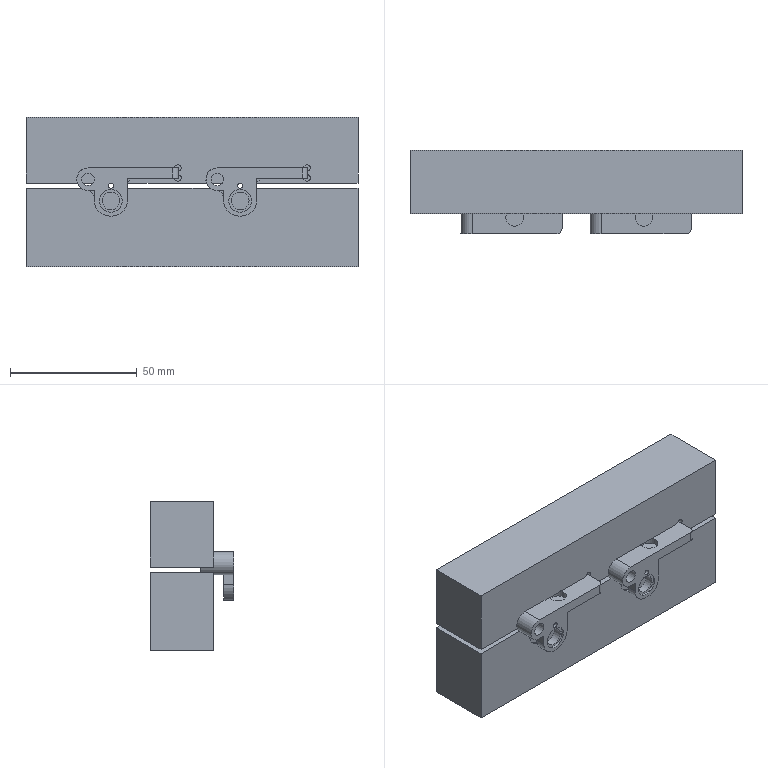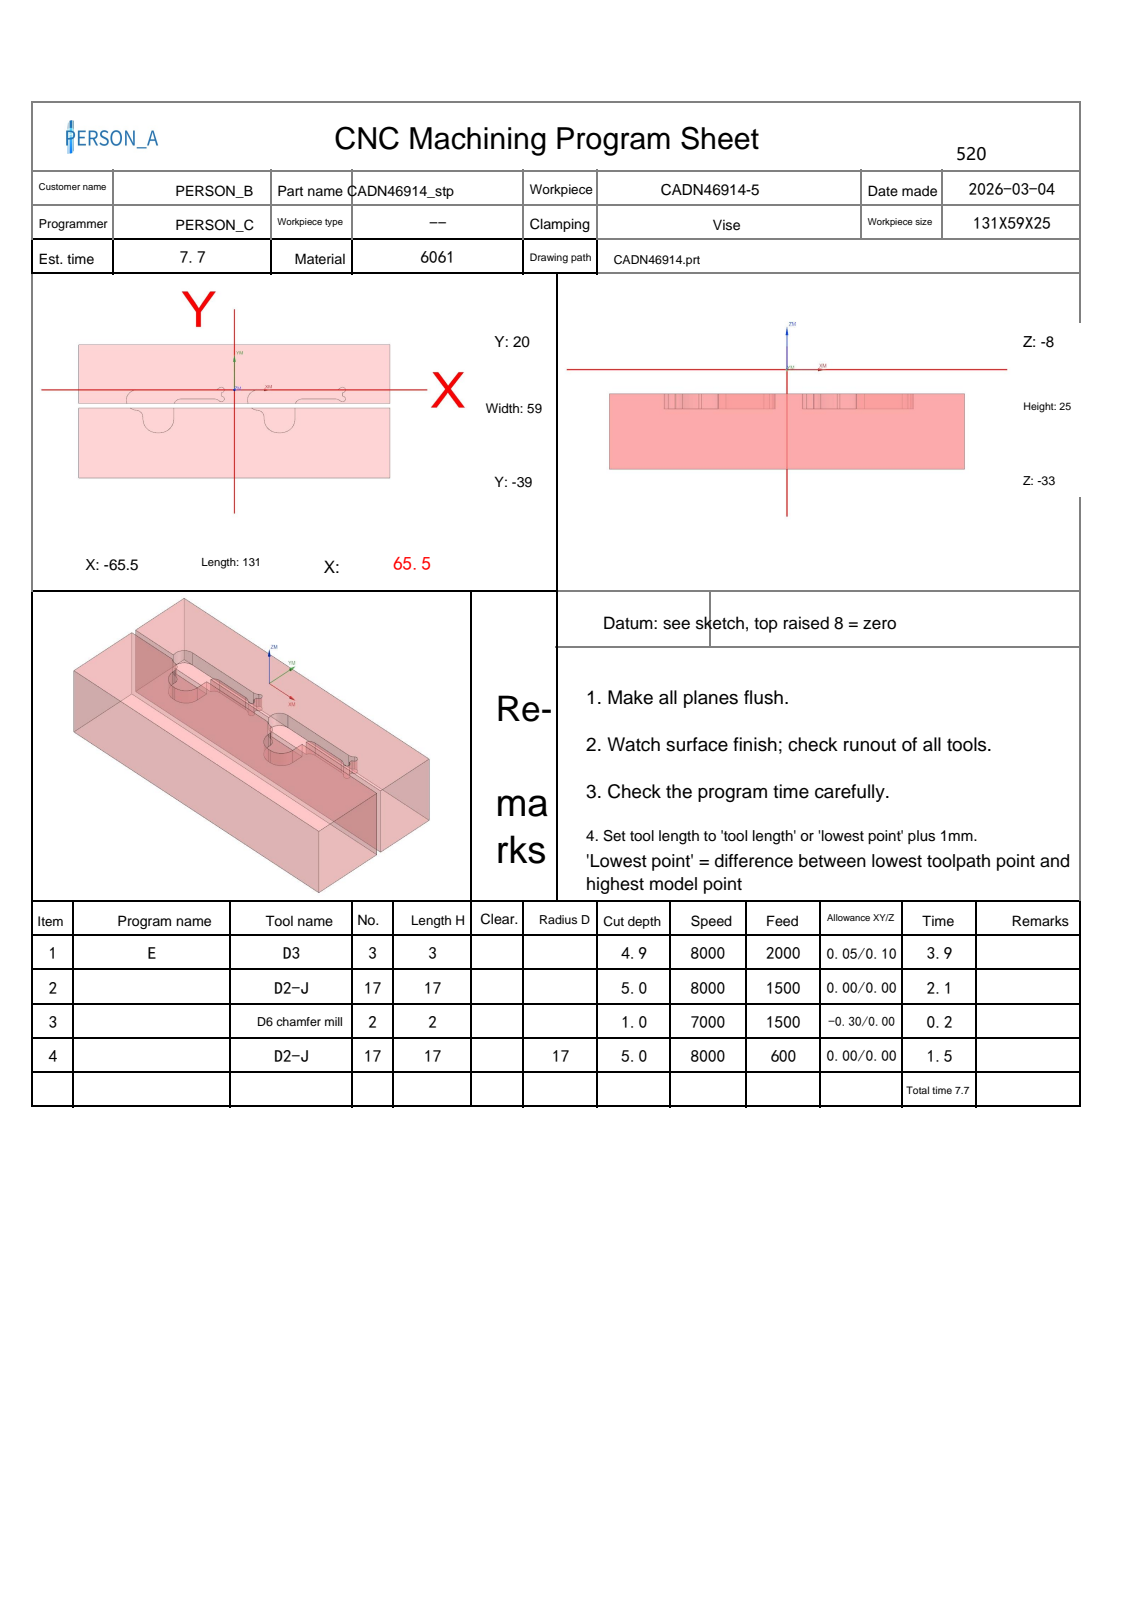NC program | NX | posted by the shop | part box 131 x 33 x 59 mm
Lines 1 to 1054 of 10523:
%
O0001
(Machine time: 8.40 MIN)
(===Total Tool:3===)
(T3=D3      D=3.   R=0.   D-  H03 Z=-12.9 )
(T17=D2-J   D=2.   R=0.   D-  H17 Z=-13.  )
(T2=D6 chamfer mill   D=6.   R=0.   D-  H02 Z=-9.   )
G80 G90 G17 G49 G40
G91 G28 Z0
M01
N1 T03 M06
(D3  D=3. R=0. H=03 ce=0.05 di=0.10)
G00 G90 G54 X-31.564 Y-11.328 M03 S8000
G43 H03 Z2.1
M08
Z-6.5
G03 X-31.564 Y-11.328 Z-6.945 I-1.336 J.192 F2000.
X-31.564 Y-11.328 Z-7.389 I-1.336 J.192
X-31.564 Y-11.328 Z-7.834 I-1.336 J.192
X-31.564 Y-11.328 Z-8.278 I-1.336 J.192
X-31.55 Y-11.136 Z-8.288 I-1.336 J.192
G01 Y-9.622
X-31.538 Y-9.552
X-31.579 Y-9.494
G02 X-32.02 Y-7.55 I4.059 J1.944
X-31.877 Y-6.424 I4.5 J0.0
G01 X-31.868 Y-6.35
G03 X-32.167 Y-6.05 I-.3 J0.0
G01 X-34.038
G03 X-34.338 Y-6.35 I.001 J-.3
G01 X-34.277 Y-6.53
G02 X-32.45 Y-11.983 I-7.223 J-5.453
G01 Y-12.651
G03 X-32.151 Y-12.95 I.3 J.001
G01 X-31.849
G03 X-31.55 Y-12.651 I-.001 J.3
G01 Y-12.047
G02 X-31.417 Y-11.797 I.3 J0.0
G01 X-29.433 Y-10.475
G03 X-29.3 Y-10.226 I-.167 J.25
G01 Y-9.025
X-29.295 Y-8.929
X-29.355 Y-8.853
G02 X-29.77 Y-7.55 I1.835 J1.303
X-29.642 Y-6.8 I2.25 J0.0
G01 X-29.183 Y-5.502
X-29.15 Y-5.439
X-29.154 Y-5.369
X-29.196 Y-5.311
X-29.331 Y-5.049
X-29.376 Y-4.983
X-29.363 Y-4.904
Y-4.886
G03 X-30.113 Y-4.136 I-.75 J0.0
X-30.544 Y-4.272 I0.0 J-.75
G01 X-31.725 Y-5.102
G03 X-32.044 Y-5.716 I.431 J-.614
X-31.294 Y-6.466 I.75 J0.0
X-30.863 Y-6.329 I0.0 J.75
G01 X-29.682 Y-5.5
G03 X-29.512 Y-5.334 I-.431 J.614
G01 X-29.481 Y-5.274
X-29.416 Y-5.258
X-29.155 Y-5.143
G03 X-28.994 Y-4.968 I-.122 J.274
G01 X-28.911 Y-4.733
G02 X-28.707 Y-4.222 I6.411 J-2.267
G01 X-28.681 Y-4.1
G03 X-28.98 Y-3.8 I-.3 J0.0
G01 X-36.616
G03 X-36.82 Y-3.881 I0.0 J-.3
G01 X-37.21 Y-4.244
X-37.275 Y-4.313
X-37.37 Y-4.321
G03 X-38.008 Y-5.063 I.111 J-.742
X-37.505 Y-5.771 I.75 J0.0
G01 X-35.247 Y-6.558
G03 X-35. Y-6.6 I.247 J.708
X-34.25 Y-5.85 I0.0 J.75
X-34.753 Y-5.142 I-.75 J0.0
G01 X-36.671 Y-4.473
X-36.754 Y-4.453
X-36.803 Y-4.382
X-37.199 Y-3.908
G03 X-37.429 Y-3.8 I-.23 J-.192
G01 X-41.
G03 X-41.7 Y-4.5 I0.0 J-.7
X-41.66 Y-4.733 I.7 J0.0
G01 X-41.622 Y-4.841
X-41.601 Y-4.925
X-41.529 Y-4.973
X-41.44 Y-5.044
G03 X-41.047 Y-5.198 I.44 J.544
G02 X-34.7 Y-11.983 I-.453 J-6.785
G01 Y-13.
G03 X-32.5 Y-15.2 I2.2 J0.0
G01 X-31.5
G03 X-29.3 Y-13. I0.0 J2.2
G01 Y-12.047
G02 X-29.167 Y-11.797 I.3 J0.0
G01 X-27.183 Y-10.475
G03 X-27.05 Y-10.226 I-.167 J.25
G01 Y-7.55
X-27.52
X-26.79 Y-5.483
G02 X-22.5 Y-2.45 I4.29 J-1.517
G01 X-8.51
G02 X-7.05 Y-2.691 I0.0 J-4.55
G01 Y-1.309
G02 X-8.51 Y-1.55 I-1.46 J4.309
G01 X-26.738
G03 X-27.038 Y-1.85 I0.0 J-.3
G01 X-27.031 Y-1.913
X-27.025 Y-1.94
X-27.018 Y-2.004
G02 X-27.194 Y-2.277 I-.3 J0.0
G01 X-28.386 Y-2.819
G03 X-28.825 Y-3.502 I.311 J-.683
X-28.075 Y-4.252 I.75 J0.0
X-27.765 Y-4.184 I0.0 J.75
G01 X-26.117 Y-3.434
G03 X-25.677 Y-2.752 I-.311 J.683
X-26.318 Y-2.01 I-.75 J0.0
G02 X-26.544 Y-1.813 I.041 J.275
G01 X-26.589 Y-1.662
X-26.605 Y-1.591
X-26.665 Y-1.546
X-26.738 Y-1.55
X-41.
G03 X-43.95 Y-4.5 I0.0 J-2.95
X-43.781 Y-5.483 I2.95 J0.0
G01 X-43.44 Y-6.45
X-43.28
X-42.854 Y-6.794
G03 X-41.197 Y-7.443 I1.854 J2.294
G02 X-36.95 Y-11.983 I-.303 J-4.54
G01 Y-13.
G03 X-32.5 Y-17.45 I4.45 J0.0
G01 X-31.5
G03 X-27.05 Y-13. I0.0 J4.45
G01 Y-9.636
Y-9.136
X-30.05
Z-6.788
G00 X-31.564 Y-11.328
G03 X-31.564 Y-11.328 Z-7.233 I-1.336 J.192
X-31.564 Y-11.328 Z-7.677 I-1.336 J.192
X-31.564 Y-11.328 Z-8.122 I-1.336 J.192
X-31.564 Y-11.328 Z-8.566 I-1.336 J.192
X-31.55 Y-11.136 Z-8.576 I-1.336 J.192
G01 Y-9.622
X-31.538 Y-9.552
X-31.579 Y-9.494
G02 X-32.02 Y-7.55 I4.059 J1.944
X-31.877 Y-6.424 I4.5 J0.0
G01 X-31.868 Y-6.35
G03 X-32.167 Y-6.05 I-.3 J0.0
G01 X-34.038
G03 X-34.338 Y-6.35 I.001 J-.3
G01 X-34.277 Y-6.53
G02 X-32.45 Y-11.983 I-7.223 J-5.453
G01 Y-12.651
G03 X-32.151 Y-12.95 I.3 J.001
G01 X-31.849
G03 X-31.55 Y-12.651 I-.001 J.3
G01 Y-12.047
G02 X-31.417 Y-11.797 I.3 J0.0
G01 X-29.433 Y-10.475
G03 X-29.3 Y-10.226 I-.167 J.25
G01 Y-9.025
X-29.295 Y-8.929
X-29.355 Y-8.853
G02 X-29.77 Y-7.55 I1.835 J1.303
X-29.642 Y-6.8 I2.25 J0.0
G01 X-29.183 Y-5.502
X-29.15 Y-5.439
X-29.154 Y-5.369
X-29.196 Y-5.311
X-29.331 Y-5.049
X-29.376 Y-4.983
X-29.363 Y-4.904
Y-4.886
G03 X-30.113 Y-4.136 I-.75 J0.0
X-30.544 Y-4.272 I0.0 J-.75
G01 X-31.725 Y-5.102
G03 X-32.044 Y-5.716 I.431 J-.614
X-31.294 Y-6.466 I.75 J0.0
X-30.863 Y-6.329 I0.0 J.75
G01 X-29.682 Y-5.5
G03 X-29.512 Y-5.334 I-.431 J.614
G01 X-29.481 Y-5.274
X-29.416 Y-5.258
X-29.155 Y-5.143
G03 X-28.994 Y-4.968 I-.122 J.274
G01 X-28.911 Y-4.733
G02 X-28.707 Y-4.222 I6.411 J-2.267
G01 X-28.681 Y-4.1
G03 X-28.98 Y-3.8 I-.3 J0.0
G01 X-36.616
G03 X-36.82 Y-3.881 I0.0 J-.3
G01 X-37.21 Y-4.244
X-37.275 Y-4.313
X-37.37 Y-4.321
G03 X-38.008 Y-5.063 I.111 J-.742
X-37.505 Y-5.771 I.75 J0.0
G01 X-35.247 Y-6.558
G03 X-35. Y-6.6 I.247 J.708
X-34.25 Y-5.85 I0.0 J.75
X-34.753 Y-5.142 I-.75 J0.0
G01 X-36.671 Y-4.473
X-36.754 Y-4.453
X-36.803 Y-4.382
X-37.199 Y-3.908
G03 X-37.429 Y-3.8 I-.23 J-.192
G01 X-41.
G03 X-41.7 Y-4.5 I0.0 J-.7
X-41.66 Y-4.733 I.7 J0.0
G01 X-41.622 Y-4.841
X-41.601 Y-4.925
X-41.529 Y-4.973
X-41.44 Y-5.044
G03 X-41.047 Y-5.198 I.44 J.544
G02 X-34.7 Y-11.983 I-.453 J-6.785
G01 Y-13.
G03 X-32.5 Y-15.2 I2.2 J0.0
G01 X-31.5
G03 X-29.3 Y-13. I0.0 J2.2
G01 Y-12.047
G02 X-29.167 Y-11.797 I.3 J0.0
G01 X-27.183 Y-10.475
G03 X-27.05 Y-10.226 I-.167 J.25
G01 Y-7.55
X-27.52
X-26.79 Y-5.483
G02 X-22.5 Y-2.45 I4.29 J-1.517
G01 X-8.51
G02 X-7.05 Y-2.691 I0.0 J-4.55
G01 Y-1.309
G02 X-8.51 Y-1.55 I-1.46 J4.309
G01 X-26.738
G03 X-27.038 Y-1.85 I0.0 J-.3
G01 X-27.031 Y-1.913
X-27.025 Y-1.94
X-27.018 Y-2.004
G02 X-27.194 Y-2.277 I-.3 J0.0
G01 X-28.386 Y-2.819
G03 X-28.825 Y-3.502 I.311 J-.683
X-28.075 Y-4.252 I.75 J0.0
X-27.765 Y-4.184 I0.0 J.75
G01 X-26.117 Y-3.434
G03 X-25.677 Y-2.752 I-.311 J.683
X-26.318 Y-2.01 I-.75 J0.0
G02 X-26.544 Y-1.813 I.041 J.275
G01 X-26.589 Y-1.662
X-26.605 Y-1.591
X-26.665 Y-1.546
X-26.738 Y-1.55
X-41.
G03 X-43.95 Y-4.5 I0.0 J-2.95
X-43.781 Y-5.483 I2.95 J0.0
G01 X-43.44 Y-6.45
X-43.28
X-42.854 Y-6.794
G03 X-41.197 Y-7.443 I1.854 J2.294
G02 X-36.95 Y-11.983 I-.303 J-4.54
G01 Y-13.
G03 X-32.5 Y-17.45 I4.45 J0.0
G01 X-31.5
G03 X-27.05 Y-13. I0.0 J4.45
G01 Y-9.636
Y-9.136
X-30.05
Z-7.076
G00 X-31.564 Y-11.328
G03 X-31.564 Y-11.328 Z-7.521 I-1.336 J.192
X-31.564 Y-11.328 Z-7.966 I-1.336 J.192
X-31.564 Y-11.328 Z-8.41 I-1.336 J.192
X-31.564 Y-11.328 Z-8.855 I-1.336 J.192
X-31.55 Y-11.136 Z-8.865 I-1.336 J.192
G01 Y-9.622
X-31.538 Y-9.552
X-31.579 Y-9.494
G02 X-32.02 Y-7.55 I4.059 J1.944
X-31.877 Y-6.424 I4.5 J0.0
G01 X-31.868 Y-6.35
G03 X-32.167 Y-6.05 I-.3 J0.0
G01 X-34.038
G03 X-34.338 Y-6.35 I.001 J-.3
G01 X-34.277 Y-6.53
G02 X-32.45 Y-11.983 I-7.223 J-5.453
G01 Y-12.651
G03 X-32.151 Y-12.95 I.3 J.001
G01 X-31.849
G03 X-31.55 Y-12.651 I-.001 J.3
G01 Y-12.047
G02 X-31.417 Y-11.797 I.3 J0.0
G01 X-29.433 Y-10.475
G03 X-29.3 Y-10.226 I-.167 J.25
G01 Y-9.025
X-29.295 Y-8.929
X-29.355 Y-8.853
G02 X-29.77 Y-7.55 I1.835 J1.303
X-29.642 Y-6.8 I2.25 J0.0
G01 X-29.183 Y-5.502
X-29.15 Y-5.439
X-29.154 Y-5.369
X-29.196 Y-5.311
X-29.331 Y-5.049
X-29.376 Y-4.983
X-29.363 Y-4.904
Y-4.886
G03 X-30.113 Y-4.136 I-.75 J0.0
X-30.544 Y-4.272 I0.0 J-.75
G01 X-31.725 Y-5.102
G03 X-32.044 Y-5.716 I.431 J-.614
X-31.294 Y-6.466 I.75 J0.0
X-30.863 Y-6.329 I0.0 J.75
G01 X-29.682 Y-5.5
G03 X-29.512 Y-5.334 I-.431 J.614
G01 X-29.481 Y-5.274
X-29.416 Y-5.258
X-29.155 Y-5.143
G03 X-28.994 Y-4.968 I-.122 J.274
G01 X-28.911 Y-4.733
G02 X-28.707 Y-4.222 I6.411 J-2.267
G01 X-28.681 Y-4.1
G03 X-28.98 Y-3.8 I-.3 J0.0
G01 X-36.616
G03 X-36.82 Y-3.881 I0.0 J-.3
G01 X-37.21 Y-4.244
X-37.275 Y-4.313
X-37.37 Y-4.321
G03 X-38.008 Y-5.063 I.111 J-.742
X-37.505 Y-5.771 I.75 J0.0
G01 X-35.247 Y-6.558
G03 X-35. Y-6.6 I.247 J.708
X-34.25 Y-5.85 I0.0 J.75
X-34.753 Y-5.142 I-.75 J0.0
G01 X-36.671 Y-4.473
X-36.754 Y-4.453
X-36.803 Y-4.382
X-37.199 Y-3.908
G03 X-37.429 Y-3.8 I-.23 J-.192
G01 X-41.
G03 X-41.7 Y-4.5 I0.0 J-.7
X-41.66 Y-4.733 I.7 J0.0
G01 X-41.622 Y-4.841
X-41.601 Y-4.925
X-41.529 Y-4.973
X-41.44 Y-5.044
G03 X-41.047 Y-5.198 I.44 J.544
G02 X-34.7 Y-11.983 I-.453 J-6.785
G01 Y-13.
G03 X-32.5 Y-15.2 I2.2 J0.0
G01 X-31.5
G03 X-29.3 Y-13. I0.0 J2.2
G01 Y-12.047
G02 X-29.167 Y-11.797 I.3 J0.0
G01 X-27.183 Y-10.475
G03 X-27.05 Y-10.226 I-.167 J.25
G01 Y-7.55
X-27.52
X-26.79 Y-5.483
G02 X-22.5 Y-2.45 I4.29 J-1.517
G01 X-8.51
G02 X-7.05 Y-2.691 I0.0 J-4.55
G01 Y-1.309
G02 X-8.51 Y-1.55 I-1.46 J4.309
G01 X-26.738
G03 X-27.038 Y-1.85 I0.0 J-.3
G01 X-27.031 Y-1.913
X-27.025 Y-1.94
X-27.018 Y-2.004
G02 X-27.194 Y-2.277 I-.3 J0.0
G01 X-28.386 Y-2.819
G03 X-28.825 Y-3.502 I.311 J-.683
X-28.075 Y-4.252 I.75 J0.0
X-27.765 Y-4.184 I0.0 J.75
G01 X-26.117 Y-3.434
G03 X-25.677 Y-2.752 I-.311 J.683
X-26.318 Y-2.01 I-.75 J0.0
G02 X-26.544 Y-1.813 I.041 J.275
G01 X-26.589 Y-1.662
X-26.605 Y-1.591
X-26.665 Y-1.546
X-26.738 Y-1.55
X-41.
G03 X-43.95 Y-4.5 I0.0 J-2.95
X-43.781 Y-5.483 I2.95 J0.0
G01 X-43.44 Y-6.45
X-43.28
X-42.854 Y-6.794
G03 X-41.197 Y-7.443 I1.854 J2.294
G02 X-36.95 Y-11.983 I-.303 J-4.54
G01 Y-13.
G03 X-32.5 Y-17.45 I4.45 J0.0
G01 X-31.5
G03 X-27.05 Y-13. I0.0 J4.45
G01 Y-9.636
Y-9.136
X-30.05
Z-7.365
G00 X-31.564 Y-11.328
G03 X-31.564 Y-11.328 Z-7.809 I-1.336 J.192
X-31.564 Y-11.328 Z-8.254 I-1.336 J.192
X-31.564 Y-11.328 Z-8.698 I-1.336 J.192
X-31.564 Y-11.328 Z-9.143 I-1.336 J.192
X-31.55 Y-11.136 Z-9.153 I-1.336 J.192
G01 Y-9.622
X-31.538 Y-9.552
X-31.579 Y-9.494
G02 X-32.02 Y-7.55 I4.059 J1.944
X-31.877 Y-6.424 I4.5 J0.0
G01 X-31.868 Y-6.35
G03 X-32.167 Y-6.05 I-.3 J0.0
G01 X-34.038
G03 X-34.338 Y-6.35 I.001 J-.3
G01 X-34.277 Y-6.53
G02 X-32.45 Y-11.983 I-7.223 J-5.453
G01 Y-12.651
G03 X-32.151 Y-12.95 I.3 J.001
G01 X-31.849
G03 X-31.55 Y-12.651 I-.001 J.3
G01 Y-12.047
G02 X-31.417 Y-11.797 I.3 J0.0
G01 X-29.433 Y-10.475
G03 X-29.3 Y-10.226 I-.167 J.25
G01 Y-9.025
X-29.295 Y-8.929
X-29.355 Y-8.853
G02 X-29.77 Y-7.55 I1.835 J1.303
X-29.642 Y-6.8 I2.25 J0.0
G01 X-29.183 Y-5.502
X-29.15 Y-5.439
X-29.154 Y-5.369
X-29.196 Y-5.311
X-29.331 Y-5.049
X-29.376 Y-4.983
X-29.363 Y-4.904
Y-4.886
G03 X-30.113 Y-4.136 I-.75 J0.0
X-30.544 Y-4.272 I0.0 J-.75
G01 X-31.725 Y-5.102
G03 X-32.044 Y-5.716 I.431 J-.614
X-31.294 Y-6.466 I.75 J0.0
X-30.863 Y-6.329 I0.0 J.75
G01 X-29.682 Y-5.5
G03 X-29.512 Y-5.334 I-.431 J.614
G01 X-29.481 Y-5.274
X-29.416 Y-5.258
X-29.155 Y-5.143
G03 X-28.994 Y-4.968 I-.122 J.274
G01 X-28.911 Y-4.733
G02 X-28.707 Y-4.222 I6.411 J-2.267
G01 X-28.681 Y-4.1
G03 X-28.98 Y-3.8 I-.3 J0.0
G01 X-36.616
G03 X-36.82 Y-3.881 I0.0 J-.3
G01 X-37.21 Y-4.244
X-37.275 Y-4.313
X-37.37 Y-4.321
G03 X-38.008 Y-5.063 I.111 J-.742
X-37.505 Y-5.771 I.75 J0.0
G01 X-35.247 Y-6.558
G03 X-35. Y-6.6 I.247 J.708
X-34.25 Y-5.85 I0.0 J.75
X-34.753 Y-5.142 I-.75 J0.0
G01 X-36.671 Y-4.473
X-36.754 Y-4.453
X-36.803 Y-4.382
X-37.199 Y-3.908
G03 X-37.429 Y-3.8 I-.23 J-.192
G01 X-41.
G03 X-41.7 Y-4.5 I0.0 J-.7
X-41.66 Y-4.733 I.7 J0.0
G01 X-41.622 Y-4.841
X-41.601 Y-4.925
X-41.529 Y-4.973
X-41.44 Y-5.044
G03 X-41.047 Y-5.198 I.44 J.544
G02 X-34.7 Y-11.983 I-.453 J-6.785
G01 Y-13.
G03 X-32.5 Y-15.2 I2.2 J0.0
G01 X-31.5
G03 X-29.3 Y-13. I0.0 J2.2
G01 Y-12.047
G02 X-29.167 Y-11.797 I.3 J0.0
G01 X-27.183 Y-10.475
G03 X-27.05 Y-10.226 I-.167 J.25
G01 Y-7.55
X-27.52
X-26.79 Y-5.483
G02 X-22.5 Y-2.45 I4.29 J-1.517
G01 X-8.51
G02 X-7.05 Y-2.691 I0.0 J-4.55
G01 Y-1.309
G02 X-8.51 Y-1.55 I-1.46 J4.309
G01 X-26.738
G03 X-27.038 Y-1.85 I0.0 J-.3
G01 X-27.031 Y-1.913
X-27.025 Y-1.94
X-27.018 Y-2.004
G02 X-27.194 Y-2.277 I-.3 J0.0
G01 X-28.386 Y-2.819
G03 X-28.825 Y-3.502 I.311 J-.683
X-28.075 Y-4.252 I.75 J0.0
X-27.765 Y-4.184 I0.0 J.75
G01 X-26.117 Y-3.434
G03 X-25.677 Y-2.752 I-.311 J.683
X-26.318 Y-2.01 I-.75 J0.0
G02 X-26.544 Y-1.813 I.041 J.275
G01 X-26.589 Y-1.662
X-26.605 Y-1.591
X-26.665 Y-1.546
X-26.738 Y-1.55
X-41.
G03 X-43.95 Y-4.5 I0.0 J-2.95
X-43.781 Y-5.483 I2.95 J0.0
G01 X-43.44 Y-6.45
X-43.28
X-42.854 Y-6.794
G03 X-41.197 Y-7.443 I1.854 J2.294
G02 X-36.95 Y-11.983 I-.303 J-4.54
G01 Y-13.
G03 X-32.5 Y-17.45 I4.45 J0.0
G01 X-31.5
G03 X-27.05 Y-13. I0.0 J4.45
G01 Y-9.636
Y-9.136
X-30.05
Z-7.653
G00 X-31.564 Y-11.328
G03 X-31.564 Y-11.328 Z-8.097 I-1.336 J.192
X-31.564 Y-11.328 Z-8.542 I-1.336 J.192
X-31.564 Y-11.328 Z-8.987 I-1.336 J.192
X-31.564 Y-11.328 Z-9.431 I-1.336 J.192
X-31.55 Y-11.136 Z-9.441 I-1.336 J.192
G01 Y-9.622
X-31.538 Y-9.552
X-31.579 Y-9.494
G02 X-32.02 Y-7.55 I4.059 J1.944
X-31.877 Y-6.424 I4.5 J0.0
G01 X-31.868 Y-6.35
G03 X-32.167 Y-6.05 I-.3 J0.0
G01 X-34.038
G03 X-34.338 Y-6.35 I.001 J-.3
G01 X-34.277 Y-6.53
G02 X-32.45 Y-11.983 I-7.223 J-5.453
G01 Y-12.651
G03 X-32.151 Y-12.95 I.3 J.001
G01 X-31.849
G03 X-31.55 Y-12.651 I-.001 J.3
G01 Y-12.047
G02 X-31.417 Y-11.797 I.3 J0.0
G01 X-29.433 Y-10.475
G03 X-29.3 Y-10.226 I-.167 J.25
G01 Y-9.025
X-29.295 Y-8.929
X-29.355 Y-8.853
G02 X-29.77 Y-7.55 I1.835 J1.303
X-29.642 Y-6.8 I2.25 J0.0
G01 X-29.183 Y-5.502
X-29.15 Y-5.439
X-29.154 Y-5.369
X-29.196 Y-5.311
X-29.331 Y-5.049
X-29.376 Y-4.983
X-29.363 Y-4.904
Y-4.886
G03 X-30.113 Y-4.136 I-.75 J0.0
X-30.544 Y-4.272 I0.0 J-.75
G01 X-31.725 Y-5.102
G03 X-32.044 Y-5.716 I.431 J-.614
X-31.294 Y-6.466 I.75 J0.0
X-30.863 Y-6.329 I0.0 J.75
G01 X-29.682 Y-5.5
G03 X-29.512 Y-5.334 I-.431 J.614
G01 X-29.481 Y-5.274
X-29.416 Y-5.258
X-29.155 Y-5.143
G03 X-28.994 Y-4.968 I-.122 J.274
G01 X-28.911 Y-4.733
G02 X-28.707 Y-4.222 I6.411 J-2.267
G01 X-28.681 Y-4.1
G03 X-28.98 Y-3.8 I-.3 J0.0
G01 X-36.616
G03 X-36.82 Y-3.881 I0.0 J-.3
G01 X-37.21 Y-4.244
X-37.275 Y-4.313
X-37.37 Y-4.321
G03 X-38.008 Y-5.063 I.111 J-.742
X-37.505 Y-5.771 I.75 J0.0
G01 X-35.247 Y-6.558
G03 X-35. Y-6.6 I.247 J.708
X-34.25 Y-5.85 I0.0 J.75
X-34.753 Y-5.142 I-.75 J0.0
G01 X-36.671 Y-4.473
X-36.754 Y-4.453
X-36.803 Y-4.382
X-37.199 Y-3.908
G03 X-37.429 Y-3.8 I-.23 J-.192
G01 X-41.
G03 X-41.7 Y-4.5 I0.0 J-.7
X-41.66 Y-4.733 I.7 J0.0
G01 X-41.622 Y-4.841
X-41.601 Y-4.925
X-41.529 Y-4.973
X-41.44 Y-5.044
G03 X-41.047 Y-5.198 I.44 J.544
G02 X-34.7 Y-11.983 I-.453 J-6.785
G01 Y-13.
G03 X-32.5 Y-15.2 I2.2 J0.0
G01 X-31.5
G03 X-29.3 Y-13. I0.0 J2.2
G01 Y-12.047
G02 X-29.167 Y-11.797 I.3 J0.0
G01 X-27.183 Y-10.475
G03 X-27.05 Y-10.226 I-.167 J.25
G01 Y-7.55
X-27.52
X-26.79 Y-5.483
G02 X-22.5 Y-2.45 I4.29 J-1.517
G01 X-8.51
G02 X-7.05 Y-2.691 I0.0 J-4.55
G01 Y-1.309
G02 X-8.51 Y-1.55 I-1.46 J4.309
G01 X-26.738
G03 X-27.038 Y-1.85 I0.0 J-.3
G01 X-27.031 Y-1.913
X-27.025 Y-1.94
X-27.018 Y-2.004
G02 X-27.194 Y-2.277 I-.3 J0.0
G01 X-28.386 Y-2.819
G03 X-28.825 Y-3.502 I.311 J-.683
X-28.075 Y-4.252 I.75 J0.0
X-27.765 Y-4.184 I0.0 J.75
G01 X-26.117 Y-3.434
G03 X-25.677 Y-2.752 I-.311 J.683
X-26.318 Y-2.01 I-.75 J0.0
G02 X-26.544 Y-1.813 I.041 J.275
G01 X-26.589 Y-1.662
X-26.605 Y-1.591
X-26.665 Y-1.546
X-26.738 Y-1.55
X-41.
G03 X-43.95 Y-4.5 I0.0 J-2.95
X-43.781 Y-5.483 I2.95 J0.0
G01 X-43.44 Y-6.45
X-43.28
X-42.854 Y-6.794
G03 X-41.197 Y-7.443 I1.854 J2.294
G02 X-36.95 Y-11.983 I-.303 J-4.54
G01 Y-13.
G03 X-32.5 Y-17.45 I4.45 J0.0
G01 X-31.5
G03 X-27.05 Y-13. I0.0 J4.45
G01 Y-9.636
Y-9.136
X-30.05
Z-7.941
G00 X-31.564 Y-11.328
G03 X-31.564 Y-11.328 Z-8.386 I-1.336 J.192
X-31.564 Y-11.328 Z-8.83 I-1.336 J.192
X-31.564 Y-11.328 Z-9.275 I-1.336 J.192
X-31.564 Y-11.328 Z-9.719 I-1.336 J.192
X-31.55 Y-11.136 Z-9.729 I-1.336 J.192
G01 Y-9.622
X-31.538 Y-9.552
X-31.579 Y-9.494
G02 X-32.02 Y-7.55 I4.059 J1.944
X-31.877 Y-6.424 I4.5 J0.0
G01 X-31.868 Y-6.35
G03 X-32.167 Y-6.05 I-.3 J0.0
G01 X-34.038
G03 X-34.338 Y-6.35 I.001 J-.3
G01 X-34.277 Y-6.53
G02 X-32.45 Y-11.983 I-7.223 J-5.453
G01 Y-12.651
G03 X-32.151 Y-12.95 I.3 J.001
G01 X-31.849
G03 X-31.55 Y-12.651 I-.001 J.3
G01 Y-12.047
G02 X-31.417 Y-11.797 I.3 J0.0
G01 X-29.433 Y-10.475
G03 X-29.3 Y-10.226 I-.167 J.25
G01 Y-9.025
X-29.295 Y-8.929
X-29.355 Y-8.853
G02 X-29.77 Y-7.55 I1.835 J1.303
X-29.642 Y-6.8 I2.25 J0.0
G01 X-29.183 Y-5.502
X-29.15 Y-5.439
X-29.154 Y-5.369
X-29.196 Y-5.311
X-29.331 Y-5.049
X-29.376 Y-4.983
X-29.363 Y-4.904
Y-4.886
G03 X-30.113 Y-4.136 I-.75 J0.0
X-30.544 Y-4.272 I0.0 J-.75
G01 X-31.725 Y-5.102
G03 X-32.044 Y-5.716 I.431 J-.614
X-31.294 Y-6.466 I.75 J0.0
X-30.863 Y-6.329 I0.0 J.75
G01 X-29.682 Y-5.5
G03 X-29.512 Y-5.334 I-.431 J.614
G01 X-29.481 Y-5.274
X-29.416 Y-5.258
X-29.155 Y-5.143
G03 X-28.994 Y-4.968 I-.122 J.274
G01 X-28.911 Y-4.733
G02 X-28.707 Y-4.222 I6.411 J-2.267
G01 X-28.681 Y-4.1
G03 X-28.98 Y-3.8 I-.3 J0.0
G01 X-36.616
G03 X-36.82 Y-3.881 I0.0 J-.3
G01 X-37.21 Y-4.244
X-37.275 Y-4.313
X-37.37 Y-4.321
G03 X-38.008 Y-5.063 I.111 J-.742
X-37.505 Y-5.771 I.75 J0.0
G01 X-35.247 Y-6.558
G03 X-35. Y-6.6 I.247 J.708
X-34.25 Y-5.85 I0.0 J.75
X-34.753 Y-5.142 I-.75 J0.0
G01 X-36.671 Y-4.473
X-36.754 Y-4.453
X-36.803 Y-4.382
X-37.199 Y-3.908
G03 X-37.429 Y-3.8 I-.23 J-.192
G01 X-41.
G03 X-41.7 Y-4.5 I0.0 J-.7
X-41.66 Y-4.733 I.7 J0.0
G01 X-41.622 Y-4.841
X-41.601 Y-4.925
X-41.529 Y-4.973
X-41.44 Y-5.044
G03 X-41.047 Y-5.198 I.44 J.544
G02 X-34.7 Y-11.983 I-.453 J-6.785
G01 Y-13.
G03 X-32.5 Y-15.2 I2.2 J0.0
G01 X-31.5
G03 X-29.3 Y-13. I0.0 J2.2
G01 Y-12.047
G02 X-29.167 Y-11.797 I.3 J0.0
G01 X-27.183 Y-10.475
G03 X-27.05 Y-10.226 I-.167 J.25
G01 Y-7.55
X-27.52
X-26.79 Y-5.483
G02 X-22.5 Y-2.45 I4.29 J-1.517
G01 X-8.51
G02 X-7.05 Y-2.691 I0.0 J-4.55
G01 Y-1.309
G02 X-8.51 Y-1.55 I-1.46 J4.309
G01 X-26.738
G03 X-27.038 Y-1.85 I0.0 J-.3
G01 X-27.031 Y-1.913
X-27.025 Y-1.94
X-27.018 Y-2.004
G02 X-27.194 Y-2.277 I-.3 J0.0
G01 X-28.386 Y-2.819
G03 X-28.825 Y-3.502 I.311 J-.683
X-28.075 Y-4.252 I.75 J0.0
X-27.765 Y-4.184 I0.0 J.75
G01 X-26.117 Y-3.434
G03 X-25.677 Y-2.752 I-.311 J.683
X-26.318 Y-2.01 I-.75 J0.0
G02 X-26.544 Y-1.813 I.041 J.275
G01 X-26.589 Y-1.662
X-26.605 Y-1.591
X-26.665 Y-1.546
X-26.738 Y-1.55
X-41.
G03 X-43.95 Y-4.5 I0.0 J-2.95
X-43.781 Y-5.483 I2.95 J0.0
G01 X-43.44 Y-6.45
X-43.28
X-42.854 Y-6.794
G03 X-41.197 Y-7.443 I1.854 J2.294
G02 X-36.95 Y-11.983 I-.303 J-4.54
G01 Y-13.
G03 X-32.5 Y-17.45 I4.45 J0.0
G01 X-31.5
G03 X-27.05 Y-13. I0.0 J4.45
G01 Y-9.636
Y-9.136
X-30.05
Z-8.229
G00 X-31.564 Y-11.328
G03 X-31.564 Y-11.328 Z-8.674 I-1.336 J.192
X-31.564 Y-11.328 Z-9.118 I-1.336 J.192
X-31.564 Y-11.328 Z-9.563 I-1.336 J.192
X-31.564 Y-11.328 Z-10.008 I-1.336 J.192
X-31.55 Y-11.136 Z-10.018 I-1.336 J.192
G01 Y-9.622
X-31.538 Y-9.552
X-31.579 Y-9.494
G02 X-32.02 Y-7.55 I4.059 J1.944
X-31.877 Y-6.424 I4.5 J0.0
G01 X-31.868 Y-6.35
G03 X-32.167 Y-6.05 I-.3 J0.0
G01 X-34.038
G03 X-34.338 Y-6.35 I.001 J-.3
G01 X-34.277 Y-6.53
G02 X-32.45 Y-11.983 I-7.223 J-5.453
G01 Y-12.651
G03 X-32.151 Y-12.95 I.3 J.001
G01 X-31.849
G03 X-31.55 Y-12.651 I-.001 J.3
G01 Y-12.047
G02 X-31.417 Y-11.797 I.3 J0.0
G01 X-29.433 Y-10.475
G03 X-29.3 Y-10.226 I-.167 J.25
G01 Y-9.025
X-29.295 Y-8.929
X-29.355 Y-8.853
G02 X-29.77 Y-7.55 I1.835 J1.303
X-29.642 Y-6.8 I2.25 J0.0
G01 X-29.183 Y-5.502
X-29.15 Y-5.439
X-29.154 Y-5.369
X-29.196 Y-5.311
X-29.331 Y-5.049
X-29.376 Y-4.983
X-29.363 Y-4.904
Y-4.886
G03 X-30.113 Y-4.136 I-.75 J0.0
X-30.544 Y-4.272 I0.0 J-.75
G01 X-31.725 Y-5.102
G03 X-32.044 Y-5.716 I.431 J-.614
X-31.294 Y-6.466 I.75 J0.0
X-30.863 Y-6.329 I0.0 J.75
G01 X-29.682 Y-5.5
G03 X-29.512 Y-5.334 I-.431 J.614
G01 X-29.481 Y-5.274
X-29.416 Y-5.258
X-29.155 Y-5.143
G03 X-28.994 Y-4.968 I-.122 J.274
G01 X-28.911 Y-4.733
G02 X-28.707 Y-4.222 I6.411 J-2.267
G01 X-28.681 Y-4.1
G03 X-28.98 Y-3.8 I-.3 J0.0
G01 X-36.616
G03 X-36.82 Y-3.881 I0.0 J-.3
G01 X-37.21 Y-4.244
X-37.275 Y-4.313
X-37.37 Y-4.321
G03 X-38.008 Y-5.063 I.111 J-.742
X-37.505 Y-5.771 I.75 J0.0
G01 X-35.247 Y-6.558
G03 X-35. Y-6.6 I.247 J.708
X-34.25 Y-5.85 I0.0 J.75
X-34.753 Y-5.142 I-.75 J0.0
G01 X-36.671 Y-4.473
X-36.754 Y-4.453
X-36.803 Y-4.382
X-37.199 Y-3.908
G03 X-37.429 Y-3.8 I-.23 J-.192
G01 X-41.
G03 X-41.7 Y-4.5 I0.0 J-.7
X-41.66 Y-4.733 I.7 J0.0
G01 X-41.622 Y-4.841
X-41.601 Y-4.925
X-41.529 Y-4.973
X-41.44 Y-5.044
G03 X-41.047 Y-5.198 I.44 J.544
G02 X-34.7 Y-11.983 I-.453 J-6.785
G01 Y-13.
G03 X-32.5 Y-15.2 I2.2 J0.0
G01 X-31.5
G03 X-29.3 Y-13. I0.0 J2.2
G01 Y-12.047
G02 X-29.167 Y-11.797 I.3 J0.0
G01 X-27.183 Y-10.475
G03 X-27.05 Y-10.226 I-.167 J.25
G01 Y-7.55
X-27.52
X-26.79 Y-5.483
G02 X-22.5 Y-2.45 I4.29 J-1.517
G01 X-8.51
G02 X-7.05 Y-2.691 I0.0 J-4.55
G01 Y-1.309
G02 X-8.51 Y-1.55 I-1.46 J4.309
G01 X-26.738
G03 X-27.038 Y-1.85 I0.0 J-.3
G01 X-27.031 Y-1.913
X-27.025 Y-1.94
X-27.018 Y-2.004
G02 X-27.194 Y-2.277 I-.3 J0.0
G01 X-28.386 Y-2.819
G03 X-28.825 Y-3.502 I.311 J-.683
X-28.075 Y-4.252 I.75 J0.0
X-27.765 Y-4.184 I0.0 J.75
G01 X-26.117 Y-3.434
G03 X-25.677 Y-2.752 I-.311 J.683
X-26.318 Y-2.01 I-.75 J0.0
G02 X-26.544 Y-1.813 I.041 J.275
G01 X-26.589 Y-1.662
X-26.605 Y-1.591
X-26.665 Y-1.546
X-26.738 Y-1.55
X-41.
G03 X-43.95 Y-4.5 I0.0 J-2.95
X-43.781 Y-5.483 I2.95 J0.0
G01 X-43.44 Y-6.45
X-43.28
X-42.854 Y-6.794
G03 X-41.197 Y-7.443 I1.854 J2.294
G02 X-36.95 Y-11.983 I-.303 J-4.54
G01 Y-13.
G03 X-32.5 Y-17.45 I4.45 J0.0
G01 X-31.5
G03 X-27.05 Y-13. I0.0 J4.45
G01 Y-9.636
Y-9.136
X-30.05
Z-8.518
G00 X-31.564 Y-11.328
G03 X-31.564 Y-11.328 Z-8.962 I-1.336 J.192
X-31.564 Y-11.328 Z-9.407 I-1.336 J.192
X-31.564 Y-11.328 Z-9.851 I-1.336 J.192
X-31.564 Y-11.328 Z-10.296 I-1.336 J.192
X-31.55 Y-11.136 Z-10.306 I-1.336 J.192
G01 Y-9.622
X-31.538 Y-9.552
X-31.579 Y-9.494
G02 X-32.02 Y-7.55 I4.059 J1.944
X-31.877 Y-6.424 I4.5 J0.0
G01 X-31.868 Y-6.35
G03 X-32.167 Y-6.05 I-.3 J0.0
G01 X-34.038
G03 X-34.338 Y-6.35 I.001 J-.3
G01 X-34.277 Y-6.53
G02 X-32.45 Y-11.983 I-7.223 J-5.453
G01 Y-12.651
G03 X-32.151 Y-12.95 I.3 J.001
G01 X-31.849
G03 X-31.55 Y-12.651 I-.001 J.3
G01 Y-12.047
G02 X-31.417 Y-11.797 I.3 J0.0
G01 X-29.433 Y-10.475
G03 X-29.3 Y-10.226 I-.167 J.25
G01 Y-9.025
X-29.295 Y-8.929
X-29.355 Y-8.853
G02 X-29.77 Y-7.55 I1.835 J1.303
X-29.642 Y-6.8 I2.25 J0.0
G01 X-29.183 Y-5.502
X-29.15 Y-5.439
X-29.154 Y-5.369
X-29.196 Y-5.311
X-29.331 Y-5.049
X-29.376 Y-4.983
X-29.363 Y-4.904
Y-4.886
G03 X-30.113 Y-4.136 I-.75 J0.0
X-30.544 Y-4.272 I0.0 J-.75
G01 X-31.725 Y-5.102
G03 X-32.044 Y-5.716 I.431 J-.614
X-31.294 Y-6.466 I.75 J0.0
X-30.863 Y-6.329 I0.0 J.75
G01 X-29.682 Y-5.5
G03 X-29.512 Y-5.334 I-.431 J.614
G01 X-29.481 Y-5.274
X-29.416 Y-5.258
X-29.155 Y-5.143
G03 X-28.994 Y-4.968 I-.122 J.274
G01 X-28.911 Y-4.733
G02 X-28.707 Y-4.222 I6.411 J-2.267
G01 X-28.681 Y-4.1
G03 X-28.98 Y-3.8 I-.3 J0.0
G01 X-36.616
G03 X-36.82 Y-3.881 I0.0 J-.3
G01 X-37.21 Y-4.244
X-37.275 Y-4.313
X-37.37 Y-4.321
G03 X-38.008 Y-5.063 I.111 J-.742
X-37.505 Y-5.771 I.75 J0.0
G01 X-35.247 Y-6.558
G03 X-35. Y-6.6 I.247 J.708
X-34.25 Y-5.85 I0.0 J.75
X-34.753 Y-5.142 I-.75 J0.0
G01 X-36.671 Y-4.473
X-36.754 Y-4.453
X-36.803 Y-4.382
X-37.199 Y-3.908
G03 X-37.429 Y-3.8 I-.23 J-.192
G01 X-41.
G03 X-41.7 Y-4.5 I0.0 J-.7
X-41.66 Y-4.733 I.7 J0.0
G01 X-41.622 Y-4.841
X-41.601 Y-4.925
X-41.529 Y-4.973
X-41.44 Y-5.044
G03 X-41.047 Y-5.198 I.44 J.544
G02 X-34.7 Y-11.983 I-.453 J-6.785
G01 Y-13.
G03 X-32.5 Y-15.2 I2.2 J0.0
G01 X-31.5
G03 X-29.3 Y-13. I0.0 J2.2
G01 Y-12.047
G02 X-29.167 Y-11.797 I.3 J0.0
G01 X-27.183 Y-10.475
G03 X-27.05 Y-10.226 I-.167 J.25
G01 Y-7.55
X-27.52
X-26.79 Y-5.483
G02 X-22.5 Y-2.45 I4.29 J-1.517
G01 X-8.51
G02 X-7.05 Y-2.691 I0.0 J-4.55
G01 Y-1.309
G02 X-8.51 Y-1.55 I-1.46 J4.309
G01 X-26.738
G03 X-27.038 Y-1.85 I0.0 J-.3
G01 X-27.031 Y-1.913
X-27.025 Y-1.94
X-27.018 Y-2.004
G02 X-27.194 Y-2.277 I-.3 J0.0
G01 X-28.386 Y-2.819
G03 X-28.825 Y-3.502 I.311 J-.683
X-28.075 Y-4.252 I.75 J0.0
X-27.765 Y-4.184 I0.0 J.75
G01 X-26.117 Y-3.434
G03 X-25.677 Y-2.752 I-.311 J.683
X-26.318 Y-2.01 I-.75 J0.0
G02 X-26.544 Y-1.813 I.041 J.275
G01 X-26.589 Y-1.662
X-26.605 Y-1.591
X-26.665 Y-1.546
X-26.738 Y-1.55
X-41.
G03 X-43.95 Y-4.5 I0.0 J-2.95
X-43.781 Y-5.483 I2.95 J0.0
G01 X-43.44 Y-6.45
X-43.28
X-42.854 Y-6.794
G03 X-41.197 Y-7.443 I1.854 J2.294
G02 X-36.95 Y-11.983 I-.303 J-4.54
G01 Y-13.
G03 X-32.5 Y-17.45 I4.45 J0.0
G01 X-31.5
G03 X-27.05 Y-13. I0.0 J4.45
G01 Y-9.636
Y-9.136
X-30.05
Z-8.806
G00 X-31.564 Y-11.328
G03 X-31.564 Y-11.328 Z-9.25 I-1.336 J.192
X-31.564 Y-11.328 Z-9.695 I-1.336 J.192
X-31.564 Y-11.328 Z-10.139 I-1.336 J.192
X-31.564 Y-11.328 Z-10.584 I-1.336 J.192